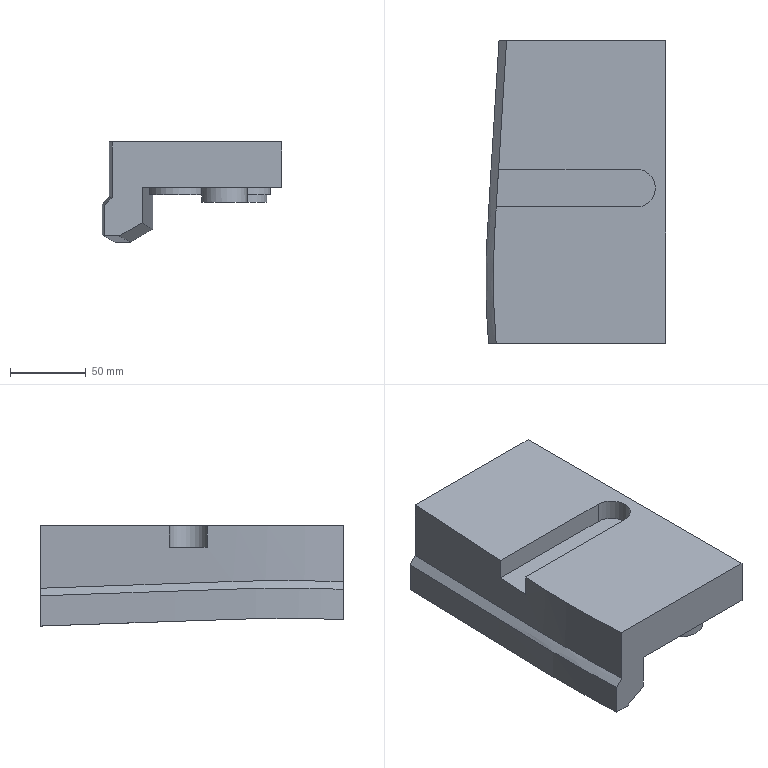Part | NX | features solid 2 | 1 solid | 25 faces | box 119.097 x 200 x 66.187 mm | volume 799855 mm3 | plane 13 | spline 6 | cylinder 6 | commonest cylinder face diameters 35 x3 30 x2 25 x1